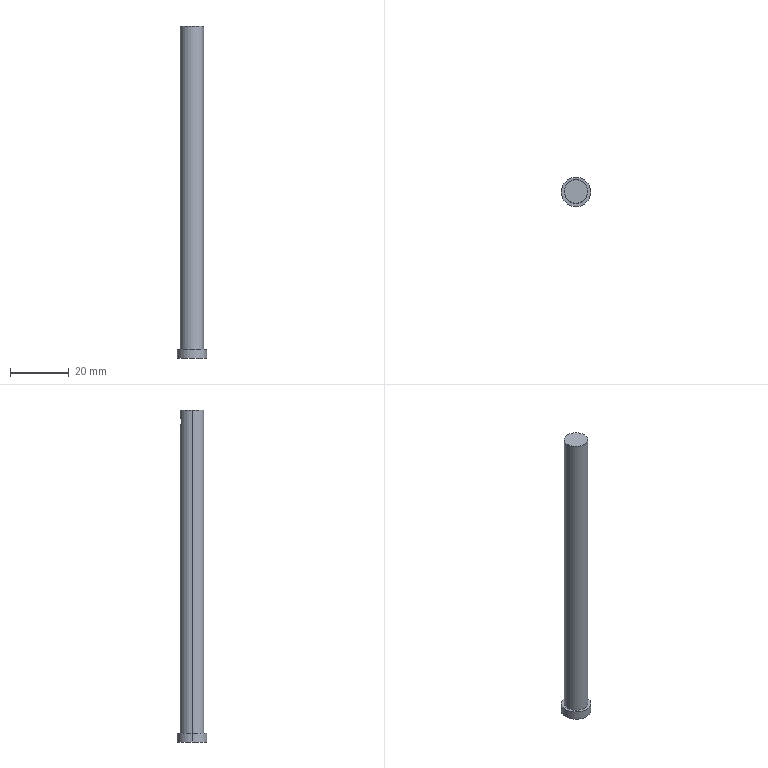Part | SolidWorks | features Extrusion 1, HoleWzd 1, ICE 1 | 1 solid | 10 faces | box 10 x 10 x 113 mm | volume 5731 mm3 | cylinder 6 | plane 4 | commonest cylinder face diameters 3.3 x2 8 x2 10 x2
STEP:
#1=CARTESIAN_POINT('',(0.,4.,107.65));
#2=VERTEX_POINT('',#1);
#3=CARTESIAN_POINT('',(0.,4.,104.35));
#4=VERTEX_POINT('',#3);
#5=CARTESIAN_POINT('',(0.,4.,107.65));
#6=CARTESIAN_POINT('',(-0.1086,4.,107.65));
#7=CARTESIAN_POINT('',(-0.2188,3.995,107.639));
#8=CARTESIAN_POINT('',(-0.4326,3.978,107.596));
#9=CARTESIAN_POINT('',(-0.5359,3.965,107.564));
#10=CARTESIAN_POINT('',(-0.8355,3.917,107.439));
#11=CARTESIAN_POINT('',(-1.016,3.872,107.318));
#12=CARTESIAN_POINT('',(-1.244,3.803,107.09));
#13=CARTESIAN_POINT('',(-1.311,3.78,107.008));
#14=CARTESIAN_POINT('',(-1.43,3.736,106.83));
#15=CARTESIAN_POINT('',(-1.481,3.716,106.734));
#16=CARTESIAN_POINT('',(-1.564,3.682,106.535));
#17=CARTESIAN_POINT('',(-1.596,3.668,106.433));
#18=CARTESIAN_POINT('',(-1.639,3.649,106.22));
#19=CARTESIAN_POINT('',(-1.65,3.644,106.109));
#20=CARTESIAN_POINT('',(-1.65,3.644,105.783));
#21=CARTESIAN_POINT('',(-1.606,3.665,105.564));
#22=CARTESIAN_POINT('',(-1.482,3.716,105.266));
#23=CARTESIAN_POINT('',(-1.43,3.736,105.17));
#24=CARTESIAN_POINT('',(-1.311,3.78,104.992));
#25=CARTESIAN_POINT('',(-1.243,3.803,104.91));
#26=CARTESIAN_POINT('',(-1.092,3.849,104.758));
#27=CARTESIAN_POINT('',(-1.008,3.872,104.689));
#28=CARTESIAN_POINT('',(-0.8311,3.914,104.571));
#29=CARTESIAN_POINT('',(-0.7368,3.933,104.52));
#30=CARTESIAN_POINT('',(-0.4348,3.982,104.393));
#31=CARTESIAN_POINT('',(-0.2205,4.,104.35));
#32=CARTESIAN_POINT('',(0.,4.,104.35));
#33=B_SPLINE_CURVE_WITH_KNOTS('',3,(#5,#6,#7,#8,#9,#10,#11,#12,#13,#14,#15,#16,#17,#18,#19,#20,#21,#22,#23,#24,#25,#26,#27,#28,#29,#30,#31,#32),.UNSPECIFIED.,.F.,.F.,(4,2,2,2,2,2,2,2,2,2,2,2,2,4),(0.005218,0.005543,0.005869,0.006521,0.006847,0.007173,0.007499,0.007824,0.008476,0.008802,0.009128,0.009454,0.009779,0.01043),.UNSPECIFIED.);
#34=EDGE_CURVE('',#2,#4,#33,.T.);
#35=ORIENTED_EDGE('',*,*,#34,.F.);
#36=CARTESIAN_POINT('',(0.,0.,107.65));
#37=VERTEX_POINT('',#36);
#38=CARTESIAN_POINT('',(0.,0.,107.65));
#39=DIRECTION('',(0.,-1.,0.));
#40=VECTOR('',#39,1000.);
#41=LINE('',#38,#40);
#42=EDGE_CURVE('',#2,#37,#41,.T.);
#43=ORIENTED_EDGE('',*,*,#42,.T.);
#44=CARTESIAN_POINT('',(0.,0.,104.35));
#45=VERTEX_POINT('',#44);
#46=CARTESIAN_POINT('',(0.,0.,106.));
#47=DIRECTION('',(0.,-1.,0.));
#48=DIRECTION('',(0.,0.,-1.));
#49=AXIS2_PLACEMENT_3D('',#46,#47,#48);
#50=CIRCLE('',#49,1.65);
#51=EDGE_CURVE('',#37,#45,#50,.T.);
#52=ORIENTED_EDGE('',*,*,#51,.T.);
#53=CARTESIAN_POINT('',(0.,0.,104.35));
#54=DIRECTION('',(0.,-1.,0.));
#55=VECTOR('',#54,1000.);
#56=LINE('',#53,#55);
#57=EDGE_CURVE('',#4,#45,#56,.T.);
#58=ORIENTED_EDGE('',*,*,#57,.F.);
#59=EDGE_LOOP('',(#35,#43,#52,#58));
#60=FACE_OUTER_BOUND('',#59,.T.);
#61=CARTESIAN_POINT('',(0.,0.,106.));
#62=DIRECTION('',(0.,-1.,0.));
#63=DIRECTION('',(0.,0.,-1.));
#64=AXIS2_PLACEMENT_3D('',#61,#62,#63);
#65=CYLINDRICAL_SURFACE('',#64,1.65);
#66=ADVANCED_FACE('',(#60),#65,.F.);
#67=CARTESIAN_POINT('',(-5.,0.,-3.));
#68=VERTEX_POINT('',#67);
#69=CARTESIAN_POINT('',(5.,0.,-3.));
#70=VERTEX_POINT('',#69);
#71=CARTESIAN_POINT('',(0.,0.,-3.));
#72=DIRECTION('',(0.,0.,-1.));
#73=DIRECTION('',(-1.,0.,0.));
#74=AXIS2_PLACEMENT_3D('',#71,#72,#73);
#75=CIRCLE('',#74,5.);
#76=EDGE_CURVE('',#68,#70,#75,.T.);
#77=ORIENTED_EDGE('',*,*,#76,.F.);
#78=CARTESIAN_POINT('',(-5.,0.,0.));
#79=VERTEX_POINT('',#78);
#80=CARTESIAN_POINT('',(-5.,0.,-3.));
#81=DIRECTION('',(0.,0.,1.));
#82=VECTOR('',#81,1000.);
#83=LINE('',#80,#82);
#84=EDGE_CURVE('',#68,#79,#83,.T.);
#85=ORIENTED_EDGE('',*,*,#84,.T.);
#86=CARTESIAN_POINT('',(5.,0.,0.));
#87=VERTEX_POINT('',#86);
#88=CARTESIAN_POINT('',(0.,0.,0.));
#89=DIRECTION('',(0.,0.,-1.));
#90=DIRECTION('',(-1.,0.,0.));
#91=AXIS2_PLACEMENT_3D('',#88,#89,#90);
#92=CIRCLE('',#91,5.);
#93=EDGE_CURVE('',#79,#87,#92,.T.);
#94=ORIENTED_EDGE('',*,*,#93,.T.);
#95=CARTESIAN_POINT('',(5.,0.,-3.));
#96=DIRECTION('',(0.,0.,1.));
#97=VECTOR('',#96,1000.);
#98=LINE('',#95,#97);
#99=EDGE_CURVE('',#70,#87,#98,.T.);
#100=ORIENTED_EDGE('',*,*,#99,.F.);
#101=EDGE_LOOP('',(#77,#85,#94,#100));
#102=FACE_OUTER_BOUND('',#101,.T.);
#103=CARTESIAN_POINT('',(0.,0.,-3.));
#104=DIRECTION('',(0.,0.,1.));
#105=DIRECTION('',(1.,0.,0.));
#106=AXIS2_PLACEMENT_3D('',#103,#104,#105);
#107=CYLINDRICAL_SURFACE('',#106,5.);
#108=ADVANCED_FACE('',(#102),#107,.T.);
#109=CARTESIAN_POINT('',(0.,4.,104.35));
#110=CARTESIAN_POINT('',(0.1103,4.,104.35));
#111=CARTESIAN_POINT('',(0.2186,3.995,104.361));
#112=CARTESIAN_POINT('',(0.4313,3.978,104.404));
#113=CARTESIAN_POINT('',(0.5367,3.965,104.436));
#114=CARTESIAN_POINT('',(0.8358,3.917,104.561));
#115=CARTESIAN_POINT('',(1.017,3.872,104.684));
#116=CARTESIAN_POINT('',(1.318,3.78,104.985));
#117=CARTESIAN_POINT('',(1.44,3.733,105.166));
#118=CARTESIAN_POINT('',(1.564,3.682,105.463));
#119=CARTESIAN_POINT('',(1.596,3.668,105.568));
#120=CARTESIAN_POINT('',(1.639,3.649,105.782));
#121=CARTESIAN_POINT('',(1.65,3.644,105.89));
#122=CARTESIAN_POINT('',(1.65,3.644,106.108));
#123=CARTESIAN_POINT('',(1.639,3.649,106.219));
#124=CARTESIAN_POINT('',(1.596,3.668,106.431));
#125=CARTESIAN_POINT('',(1.565,3.682,106.535));
#126=CARTESIAN_POINT('',(1.481,3.716,106.736));
#127=CARTESIAN_POINT('',(1.43,3.736,106.83));
#128=CARTESIAN_POINT('',(1.311,3.78,107.008));
#129=CARTESIAN_POINT('',(1.242,3.803,107.092));
#130=CARTESIAN_POINT('',(1.091,3.849,107.243));
#131=CARTESIAN_POINT('',(1.009,3.872,107.31));
#132=CARTESIAN_POINT('',(0.8304,3.914,107.43));
#133=CARTESIAN_POINT('',(0.7343,3.933,107.481));
#134=CARTESIAN_POINT('',(0.4369,3.981,107.606));
#135=CARTESIAN_POINT('',(0.2174,4.,107.65));
#136=CARTESIAN_POINT('',(0.,4.,107.65));
#137=B_SPLINE_CURVE_WITH_KNOTS('',3,(#109,#110,#111,#112,#113,#114,#115,#116,#117,#118,#119,#120,#121,#122,#123,#124,#125,#126,#127,#128,#129,#130,#131,#132,#133,#134,#135,#136),.UNSPECIFIED.,.F.,.F.,(4,2,2,2,2,2,2,2,2,2,2,2,2,4),(0.,0.0003261,0.0006522,0.001304,0.001957,0.002283,0.002609,0.002935,0.003261,0.003587,0.003913,0.004239,0.004565,0.005218),.UNSPECIFIED.);
#138=EDGE_CURVE('',#4,#2,#137,.T.);
#139=ORIENTED_EDGE('',*,*,#138,.T.);
#140=ORIENTED_EDGE('',*,*,#34,.T.);
#141=EDGE_LOOP('',(#139,#140));
#142=FACE_BOUND('',#141,.T.);
#143=CARTESIAN_POINT('',(4.,0.,110.));
#144=VERTEX_POINT('',#143);
#145=CARTESIAN_POINT('',(-4.,0.,110.));
#146=VERTEX_POINT('',#145);
#147=CARTESIAN_POINT('',(0.,0.,110.));
#148=DIRECTION('',(0.,0.,1.));
#149=DIRECTION('',(1.,0.,0.));
#150=AXIS2_PLACEMENT_3D('',#147,#148,#149);
#151=CIRCLE('',#150,4.);
#152=EDGE_CURVE('',#144,#146,#151,.T.);
#153=ORIENTED_EDGE('',*,*,#152,.F.);
#154=CARTESIAN_POINT('',(4.,0.,0.));
#155=VERTEX_POINT('',#154);
#156=CARTESIAN_POINT('',(4.,0.,110.));
#157=DIRECTION('',(0.,0.,-1.));
#158=VECTOR('',#157,1000.);
#159=LINE('',#156,#158);
#160=EDGE_CURVE('',#144,#155,#159,.T.);
#161=ORIENTED_EDGE('',*,*,#160,.T.);
#162=CARTESIAN_POINT('',(-4.,0.,0.));
#163=VERTEX_POINT('',#162);
#164=CARTESIAN_POINT('',(0.,0.,0.));
#165=DIRECTION('',(0.,0.,1.));
#166=DIRECTION('',(1.,0.,0.));
#167=AXIS2_PLACEMENT_3D('',#164,#165,#166);
#168=CIRCLE('',#167,4.);
#169=EDGE_CURVE('',#155,#163,#168,.T.);
#170=ORIENTED_EDGE('',*,*,#169,.T.);
#171=CARTESIAN_POINT('',(-4.,0.,110.));
#172=DIRECTION('',(0.,0.,-1.));
#173=VECTOR('',#172,1000.);
#174=LINE('',#171,#173);
#175=EDGE_CURVE('',#146,#163,#174,.T.);
#176=ORIENTED_EDGE('',*,*,#175,.F.);
#177=EDGE_LOOP('',(#153,#161,#170,#176));
#178=FACE_OUTER_BOUND('',#177,.T.);
#179=CARTESIAN_POINT('',(0.,0.,110.));
#180=DIRECTION('',(0.,0.,-1.));
#181=DIRECTION('',(-1.,0.,0.));
#182=AXIS2_PLACEMENT_3D('',#179,#180,#181);
#183=CYLINDRICAL_SURFACE('',#182,4.);
#184=ADVANCED_FACE('',(#142,#178),#183,.T.);
#185=ORIENTED_EDGE('',*,*,#160,.F.);
#186=CARTESIAN_POINT('',(0.,0.,110.));
#187=DIRECTION('',(0.,0.,1.));
#188=DIRECTION('',(1.,0.,0.));
#189=AXIS2_PLACEMENT_3D('',#186,#187,#188);
#190=CIRCLE('',#189,4.);
#191=EDGE_CURVE('',#146,#144,#190,.T.);
#192=ORIENTED_EDGE('',*,*,#191,.F.);
#193=ORIENTED_EDGE('',*,*,#175,.T.);
#194=CARTESIAN_POINT('',(0.,0.,0.));
#195=DIRECTION('',(0.,0.,1.));
#196=DIRECTION('',(1.,0.,0.));
#197=AXIS2_PLACEMENT_3D('',#194,#195,#196);
#198=CIRCLE('',#197,4.);
#199=EDGE_CURVE('',#163,#155,#198,.T.);
#200=ORIENTED_EDGE('',*,*,#199,.T.);
#201=EDGE_LOOP('',(#185,#192,#193,#200));
#202=FACE_OUTER_BOUND('',#201,.T.);
#203=CARTESIAN_POINT('',(0.,0.,110.));
#204=DIRECTION('',(0.,0.,-1.));
#205=DIRECTION('',(-1.,0.,0.));
#206=AXIS2_PLACEMENT_3D('',#203,#204,#205);
#207=CYLINDRICAL_SURFACE('',#206,4.);
#208=ADVANCED_FACE('',(#202),#207,.T.);
#209=ORIENTED_EDGE('',*,*,#191,.T.);
#210=ORIENTED_EDGE('',*,*,#152,.T.);
#211=EDGE_LOOP('',(#209,#210));
#212=FACE_OUTER_BOUND('',#211,.T.);
#213=CARTESIAN_POINT('',(0.,0.,110.));
#214=DIRECTION('',(0.,0.,1.));
#215=DIRECTION('',(1.,0.,0.));
#216=AXIS2_PLACEMENT_3D('',#213,#214,#215);
#217=PLANE('',#216);
#218=ADVANCED_FACE('',(#212),#217,.T.);
#219=ORIENTED_EDGE('',*,*,#84,.F.);
#220=CARTESIAN_POINT('',(0.,0.,-3.));
#221=DIRECTION('',(0.,0.,-1.));
#222=DIRECTION('',(-1.,0.,0.));
#223=AXIS2_PLACEMENT_3D('',#220,#221,#222);
#224=CIRCLE('',#223,5.);
#225=EDGE_CURVE('',#70,#68,#224,.T.);
#226=ORIENTED_EDGE('',*,*,#225,.F.);
#227=ORIENTED_EDGE('',*,*,#99,.T.);
#228=CARTESIAN_POINT('',(0.,0.,0.));
#229=DIRECTION('',(0.,0.,-1.));
#230=DIRECTION('',(-1.,0.,0.));
#231=AXIS2_PLACEMENT_3D('',#228,#229,#230);
#232=CIRCLE('',#231,5.);
#233=EDGE_CURVE('',#87,#79,#232,.T.);
#234=ORIENTED_EDGE('',*,*,#233,.T.);
#235=EDGE_LOOP('',(#219,#226,#227,#234));
#236=FACE_OUTER_BOUND('',#235,.T.);
#237=CARTESIAN_POINT('',(0.,0.,-3.));
#238=DIRECTION('',(0.,0.,1.));
#239=DIRECTION('',(1.,0.,0.));
#240=AXIS2_PLACEMENT_3D('',#237,#238,#239);
#241=CYLINDRICAL_SURFACE('',#240,5.);
#242=ADVANCED_FACE('',(#236),#241,.T.);
#243=ORIENTED_EDGE('',*,*,#225,.T.);
#244=ORIENTED_EDGE('',*,*,#76,.T.);
#245=EDGE_LOOP('',(#243,#244));
#246=FACE_OUTER_BOUND('',#245,.T.);
#247=CARTESIAN_POINT('',(0.,0.,-3.));
#248=DIRECTION('',(0.,0.,-1.));
#249=DIRECTION('',(-1.,0.,0.));
#250=AXIS2_PLACEMENT_3D('',#247,#248,#249);
#251=PLANE('',#250);
#252=ADVANCED_FACE('',(#246),#251,.T.);
#253=ORIENTED_EDGE('',*,*,#199,.F.);
#254=ORIENTED_EDGE('',*,*,#169,.F.);
#255=EDGE_LOOP('',(#253,#254));
#256=FACE_BOUND('',#255,.T.);
#257=ORIENTED_EDGE('',*,*,#233,.F.);
#258=ORIENTED_EDGE('',*,*,#93,.F.);
#259=EDGE_LOOP('',(#257,#258));
#260=FACE_OUTER_BOUND('',#259,.T.);
#261=CARTESIAN_POINT('',(0.,0.,0.));
#262=DIRECTION('',(0.,0.,-1.));
#263=DIRECTION('',(-1.,0.,0.));
#264=AXIS2_PLACEMENT_3D('',#261,#262,#263);
#265=PLANE('',#264);
#266=ADVANCED_FACE('',(#256,#260),#265,.F.);
#267=ORIENTED_EDGE('',*,*,#42,.F.);
#268=ORIENTED_EDGE('',*,*,#138,.F.);
#269=ORIENTED_EDGE('',*,*,#57,.T.);
#270=CARTESIAN_POINT('',(0.,0.,106.));
#271=DIRECTION('',(0.,-1.,0.));
#272=DIRECTION('',(0.,0.,-1.));
#273=AXIS2_PLACEMENT_3D('',#270,#271,#272);
#274=CIRCLE('',#273,1.65);
#275=EDGE_CURVE('',#45,#37,#274,.T.);
#276=ORIENTED_EDGE('',*,*,#275,.T.);
#277=EDGE_LOOP('',(#267,#268,#269,#276));
#278=FACE_OUTER_BOUND('',#277,.T.);
#279=CARTESIAN_POINT('',(0.,0.,106.));
#280=DIRECTION('',(0.,-1.,0.));
#281=DIRECTION('',(0.,0.,-1.));
#282=AXIS2_PLACEMENT_3D('',#279,#280,#281);
#283=CYLINDRICAL_SURFACE('',#282,1.65);
#284=ADVANCED_FACE('',(#278),#283,.F.);
#285=ORIENTED_EDGE('',*,*,#275,.F.);
#286=ORIENTED_EDGE('',*,*,#51,.F.);
#287=EDGE_LOOP('',(#285,#286));
#288=FACE_OUTER_BOUND('',#287,.T.);
#289=CARTESIAN_POINT('',(1.65,0.,106.));
#290=DIRECTION('',(0.,-1.,0.));
#291=DIRECTION('',(0.,0.,-1.));
#292=AXIS2_PLACEMENT_3D('',#289,#290,#291);
#293=PLANE('',#292);
#294=ADVANCED_FACE('',(#288),#293,.F.);
#295=CLOSED_SHELL('',(#66,#108,#184,#208,#218,#242,#252,#266,#284,#294));
#296=MANIFOLD_SOLID_BREP('',#295);
#297=CARTESIAN_POINT('',(0.,0.,0.));
#298=DIRECTION('',(0.,0.,1.));
#299=DIRECTION('',(1.,0.,0.));
#300=AXIS2_PLACEMENT_3D('',#297,#298,#299);
#301=(LENGTH_UNIT()NAMED_UNIT(*)SI_UNIT(.MILLI.,.METRE.));
#302=UNCERTAINTY_MEASURE_WITH_UNIT(LENGTH_MEASURE(0.00001),#301,'','');
#303=(NAMED_UNIT(*)PLANE_ANGLE_UNIT()SI_UNIT($,.RADIAN.));
#304=(NAMED_UNIT(*)SI_UNIT($,.STERADIAN.)SOLID_ANGLE_UNIT());
#305=(GEOMETRIC_REPRESENTATION_CONTEXT(3)GLOBAL_UNCERTAINTY_ASSIGNED_CONTEXT((#302))GLOBAL_UNIT_ASSIGNED_CONTEXT((#301,#303,#304))REPRESENTATION_CONTEXT('',''));
#306=ADVANCED_BREP_SHAPE_REPRESENTATION('',(#296,#300),#305);